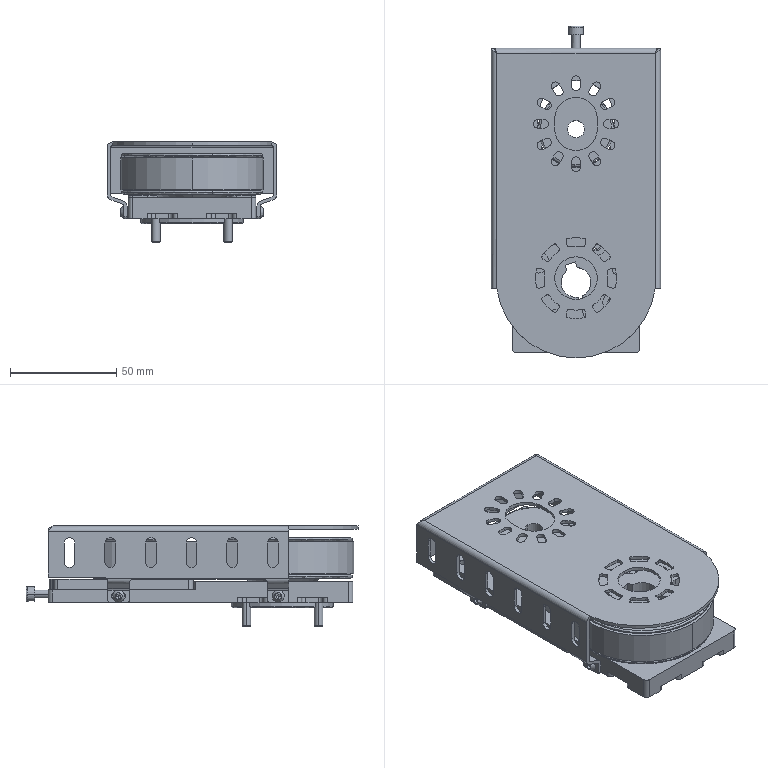Part | SolidWorks | features BaseBody 3, MoveFace 2, ICE 1 | 3 solids | 1511 faces | box 79.5 x 156 x 47 mm | volume 157908 mm3 | cylinder 860 | plane 569 | cone 48 | spline 34 | commonest cylinder face diameters 0.8 x244 2.98 x140 4 x104 63.7 x67 2 x59 5 x53